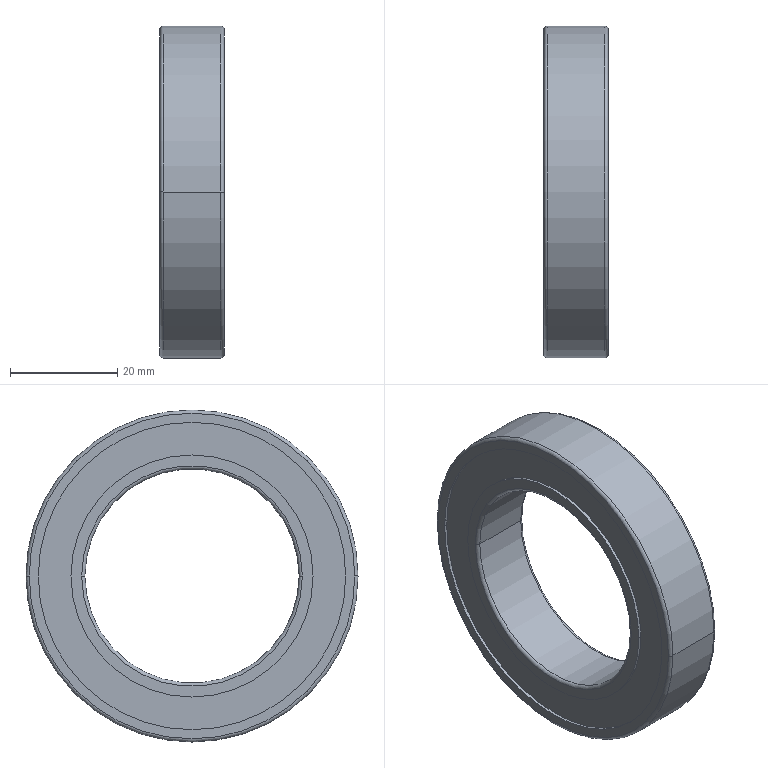Part | SolidWorks | features Fillet 2, Revolution 1 | 1 solid | 26 faces | box 12 x 62 x 62 mm | volume 20018 mm3 | cylinder 12 | torus 8 | plane 6 | commonest cylinder face diameters 45.2 x4 57.4 x4 40 x2 62 x2
STEP:
#1=CARTESIAN_POINT('',(0.6,-20.,0.));
#2=VERTEX_POINT('',#1);
#3=CARTESIAN_POINT('',(0.6,20.,0.));
#4=VERTEX_POINT('',#3);
#5=CARTESIAN_POINT('',(0.6,0.,0.));
#6=DIRECTION('',(-1.,0.,0.));
#7=DIRECTION('',(0.,1.,0.));
#8=AXIS2_PLACEMENT_3D('',#5,#6,#7);
#9=CIRCLE('',#8,20.);
#10=EDGE_CURVE('',#2,#4,#9,.T.);
#11=ORIENTED_EDGE('',*,*,#10,.F.);
#12=CARTESIAN_POINT('',(0.,-20.6,0.));
#13=VERTEX_POINT('',#12);
#14=CARTESIAN_POINT('',(0.6,-20.6,0.));
#15=DIRECTION('',(0.,0.,1.));
#16=DIRECTION('',(0.,-1.,0.));
#17=AXIS2_PLACEMENT_3D('',#14,#15,#16);
#18=CIRCLE('',#17,0.6);
#19=EDGE_CURVE('',#2,#13,#18,.T.);
#20=ORIENTED_EDGE('',*,*,#19,.T.);
#21=CARTESIAN_POINT('',(0.,20.6,0.));
#22=VERTEX_POINT('',#21);
#23=CARTESIAN_POINT('',(0.,0.,0.));
#24=DIRECTION('',(1.,0.,0.));
#25=DIRECTION('',(0.,1.,0.));
#26=AXIS2_PLACEMENT_3D('',#23,#24,#25);
#27=CIRCLE('',#26,20.6);
#28=EDGE_CURVE('',#22,#13,#27,.T.);
#29=ORIENTED_EDGE('',*,*,#28,.F.);
#30=CARTESIAN_POINT('',(0.6,20.6,0.));
#31=DIRECTION('',(0.,0.,-1.));
#32=DIRECTION('',(-1.,0.,0.));
#33=AXIS2_PLACEMENT_3D('',#30,#31,#32);
#34=CIRCLE('',#33,0.6);
#35=EDGE_CURVE('',#4,#22,#34,.T.);
#36=ORIENTED_EDGE('',*,*,#35,.F.);
#37=EDGE_LOOP('',(#11,#20,#29,#36));
#38=FACE_OUTER_BOUND('',#37,.T.);
#39=CARTESIAN_POINT('',(0.6,0.,0.));
#40=DIRECTION('',(1.,0.,0.));
#41=DIRECTION('',(0.,1.,0.));
#42=AXIS2_PLACEMENT_3D('',#39,#40,#41);
#43=TOROIDAL_SURFACE('',#42,20.6,0.6);
#44=ADVANCED_FACE('',(#38),#43,.T.);
#45=CARTESIAN_POINT('',(11.4,20.,0.));
#46=VERTEX_POINT('',#45);
#47=CARTESIAN_POINT('',(11.4,-20.,0.));
#48=VERTEX_POINT('',#47);
#49=CARTESIAN_POINT('',(11.4,0.,0.));
#50=DIRECTION('',(1.,0.,0.));
#51=DIRECTION('',(0.,-1.,0.));
#52=AXIS2_PLACEMENT_3D('',#49,#50,#51);
#53=CIRCLE('',#52,20.);
#54=EDGE_CURVE('',#46,#48,#53,.T.);
#55=ORIENTED_EDGE('',*,*,#54,.F.);
#56=CARTESIAN_POINT('',(12.,20.6,0.));
#57=VERTEX_POINT('',#56);
#58=CARTESIAN_POINT('',(11.4,20.6,0.));
#59=DIRECTION('',(0.,0.,1.));
#60=DIRECTION('',(0.,-1.,0.));
#61=AXIS2_PLACEMENT_3D('',#58,#59,#60);
#62=CIRCLE('',#61,0.6);
#63=EDGE_CURVE('',#46,#57,#62,.T.);
#64=ORIENTED_EDGE('',*,*,#63,.T.);
#65=CARTESIAN_POINT('',(12.,-20.6,0.));
#66=VERTEX_POINT('',#65);
#67=CARTESIAN_POINT('',(12.,0.,0.));
#68=DIRECTION('',(-1.,0.,0.));
#69=DIRECTION('',(0.,-1.,0.));
#70=AXIS2_PLACEMENT_3D('',#67,#68,#69);
#71=CIRCLE('',#70,20.6);
#72=EDGE_CURVE('',#66,#57,#71,.T.);
#73=ORIENTED_EDGE('',*,*,#72,.F.);
#74=CARTESIAN_POINT('',(11.4,-20.6,0.));
#75=DIRECTION('',(0.,0.,-1.));
#76=DIRECTION('',(-1.,0.,0.));
#77=AXIS2_PLACEMENT_3D('',#74,#75,#76);
#78=CIRCLE('',#77,0.6);
#79=EDGE_CURVE('',#48,#66,#78,.T.);
#80=ORIENTED_EDGE('',*,*,#79,.F.);
#81=EDGE_LOOP('',(#55,#64,#73,#80));
#82=FACE_OUTER_BOUND('',#81,.T.);
#83=CARTESIAN_POINT('',(11.4,0.,0.));
#84=DIRECTION('',(-1.,0.,0.));
#85=DIRECTION('',(0.,-1.,0.));
#86=AXIS2_PLACEMENT_3D('',#83,#84,#85);
#87=TOROIDAL_SURFACE('',#86,20.6,0.6);
#88=ADVANCED_FACE('',(#82),#87,.T.);
#89=CARTESIAN_POINT('',(0.,-30.4,0.));
#90=VERTEX_POINT('',#89);
#91=CARTESIAN_POINT('',(0.,30.4,0.));
#92=VERTEX_POINT('',#91);
#93=CARTESIAN_POINT('',(0.,0.,0.));
#94=DIRECTION('',(-1.,0.,0.));
#95=DIRECTION('',(0.,1.,0.));
#96=AXIS2_PLACEMENT_3D('',#93,#94,#95);
#97=CIRCLE('',#96,30.4);
#98=EDGE_CURVE('',#90,#92,#97,.T.);
#99=ORIENTED_EDGE('',*,*,#98,.F.);
#100=CARTESIAN_POINT('',(0.6,-31.,0.));
#101=VERTEX_POINT('',#100);
#102=CARTESIAN_POINT('',(0.6,-30.4,0.));
#103=DIRECTION('',(0.,0.,1.));
#104=DIRECTION('',(0.,-1.,0.));
#105=AXIS2_PLACEMENT_3D('',#102,#103,#104);
#106=CIRCLE('',#105,0.6);
#107=EDGE_CURVE('',#90,#101,#106,.T.);
#108=ORIENTED_EDGE('',*,*,#107,.T.);
#109=CARTESIAN_POINT('',(0.6,31.,0.));
#110=VERTEX_POINT('',#109);
#111=CARTESIAN_POINT('',(0.6,0.,0.));
#112=DIRECTION('',(1.,0.,0.));
#113=DIRECTION('',(0.,1.,0.));
#114=AXIS2_PLACEMENT_3D('',#111,#112,#113);
#115=CIRCLE('',#114,31.);
#116=EDGE_CURVE('',#110,#101,#115,.T.);
#117=ORIENTED_EDGE('',*,*,#116,.F.);
#118=CARTESIAN_POINT('',(0.6,30.4,0.));
#119=DIRECTION('',(0.,0.,-1.));
#120=DIRECTION('',(-1.,0.,0.));
#121=AXIS2_PLACEMENT_3D('',#118,#119,#120);
#122=CIRCLE('',#121,0.6);
#123=EDGE_CURVE('',#92,#110,#122,.T.);
#124=ORIENTED_EDGE('',*,*,#123,.F.);
#125=EDGE_LOOP('',(#99,#108,#117,#124));
#126=FACE_OUTER_BOUND('',#125,.T.);
#127=CARTESIAN_POINT('',(0.6,0.,0.));
#128=DIRECTION('',(1.,0.,0.));
#129=DIRECTION('',(0.,1.,0.));
#130=AXIS2_PLACEMENT_3D('',#127,#128,#129);
#131=TOROIDAL_SURFACE('',#130,30.4,0.6);
#132=ADVANCED_FACE('',(#126),#131,.T.);
#133=CARTESIAN_POINT('',(12.,30.4,0.));
#134=VERTEX_POINT('',#133);
#135=CARTESIAN_POINT('',(12.,-30.4,0.));
#136=VERTEX_POINT('',#135);
#137=CARTESIAN_POINT('',(12.,0.,0.));
#138=DIRECTION('',(1.,0.,0.));
#139=DIRECTION('',(0.,-1.,0.));
#140=AXIS2_PLACEMENT_3D('',#137,#138,#139);
#141=CIRCLE('',#140,30.4);
#142=EDGE_CURVE('',#134,#136,#141,.T.);
#143=ORIENTED_EDGE('',*,*,#142,.F.);
#144=CARTESIAN_POINT('',(11.4,31.,0.));
#145=VERTEX_POINT('',#144);
#146=CARTESIAN_POINT('',(11.4,30.4,0.));
#147=DIRECTION('',(0.,0.,1.));
#148=DIRECTION('',(0.,-1.,0.));
#149=AXIS2_PLACEMENT_3D('',#146,#147,#148);
#150=CIRCLE('',#149,0.6);
#151=EDGE_CURVE('',#134,#145,#150,.T.);
#152=ORIENTED_EDGE('',*,*,#151,.T.);
#153=CARTESIAN_POINT('',(11.4,-31.,0.));
#154=VERTEX_POINT('',#153);
#155=CARTESIAN_POINT('',(11.4,0.,0.));
#156=DIRECTION('',(-1.,0.,0.));
#157=DIRECTION('',(0.,-1.,0.));
#158=AXIS2_PLACEMENT_3D('',#155,#156,#157);
#159=CIRCLE('',#158,31.);
#160=EDGE_CURVE('',#154,#145,#159,.T.);
#161=ORIENTED_EDGE('',*,*,#160,.F.);
#162=CARTESIAN_POINT('',(11.4,-30.4,0.));
#163=DIRECTION('',(0.,0.,-1.));
#164=DIRECTION('',(-1.,0.,0.));
#165=AXIS2_PLACEMENT_3D('',#162,#163,#164);
#166=CIRCLE('',#165,0.6);
#167=EDGE_CURVE('',#136,#154,#166,.T.);
#168=ORIENTED_EDGE('',*,*,#167,.F.);
#169=EDGE_LOOP('',(#143,#152,#161,#168));
#170=FACE_OUTER_BOUND('',#169,.T.);
#171=CARTESIAN_POINT('',(11.4,0.,0.));
#172=DIRECTION('',(-1.,0.,0.));
#173=DIRECTION('',(0.,-1.,0.));
#174=AXIS2_PLACEMENT_3D('',#171,#172,#173);
#175=TOROIDAL_SURFACE('',#174,30.4,0.6);
#176=ADVANCED_FACE('',(#170),#175,.T.);
#177=ORIENTED_EDGE('',*,*,#160,.T.);
#178=CARTESIAN_POINT('',(0.,31.,0.));
#179=DIRECTION('',(-1.,0.,0.));
#180=VECTOR('',#179,1000.);
#181=LINE('',#178,#180);
#182=EDGE_CURVE('',#145,#110,#181,.T.);
#183=ORIENTED_EDGE('',*,*,#182,.T.);
#184=ORIENTED_EDGE('',*,*,#116,.T.);
#185=CARTESIAN_POINT('',(0.,-31.,0.));
#186=DIRECTION('',(-1.,0.,0.));
#187=VECTOR('',#186,1000.);
#188=LINE('',#185,#187);
#189=EDGE_CURVE('',#154,#101,#188,.T.);
#190=ORIENTED_EDGE('',*,*,#189,.F.);
#191=EDGE_LOOP('',(#177,#183,#184,#190));
#192=FACE_OUTER_BOUND('',#191,.T.);
#193=CARTESIAN_POINT('',(0.,0.,0.));
#194=DIRECTION('',(-1.,0.,0.));
#195=DIRECTION('',(0.,-1.,0.));
#196=AXIS2_PLACEMENT_3D('',#193,#194,#195);
#197=CYLINDRICAL_SURFACE('',#196,31.);
#198=ADVANCED_FACE('',(#192),#197,.T.);
#199=CARTESIAN_POINT('',(12.,28.7,0.));
#200=VERTEX_POINT('',#199);
#201=CARTESIAN_POINT('',(12.,-28.7,0.));
#202=VERTEX_POINT('',#201);
#203=CARTESIAN_POINT('',(12.,0.,0.));
#204=DIRECTION('',(-1.,0.,0.));
#205=DIRECTION('',(0.,-1.,0.));
#206=AXIS2_PLACEMENT_3D('',#203,#204,#205);
#207=CIRCLE('',#206,28.7);
#208=EDGE_CURVE('',#200,#202,#207,.T.);
#209=ORIENTED_EDGE('',*,*,#208,.F.);
#210=CARTESIAN_POINT('',(11.45,28.7,0.));
#211=VERTEX_POINT('',#210);
#212=CARTESIAN_POINT('',(0.,28.7,0.));
#213=DIRECTION('',(-1.,0.,0.));
#214=VECTOR('',#213,1000.);
#215=LINE('',#212,#214);
#216=EDGE_CURVE('',#200,#211,#215,.T.);
#217=ORIENTED_EDGE('',*,*,#216,.T.);
#218=CARTESIAN_POINT('',(11.45,-28.7,0.));
#219=VERTEX_POINT('',#218);
#220=CARTESIAN_POINT('',(11.45,0.,0.));
#221=DIRECTION('',(-1.,0.,0.));
#222=DIRECTION('',(0.,-1.,0.));
#223=AXIS2_PLACEMENT_3D('',#220,#221,#222);
#224=CIRCLE('',#223,28.7);
#225=EDGE_CURVE('',#211,#219,#224,.T.);
#226=ORIENTED_EDGE('',*,*,#225,.T.);
#227=CARTESIAN_POINT('',(0.,-28.7,0.));
#228=DIRECTION('',(-1.,0.,0.));
#229=VECTOR('',#228,1000.);
#230=LINE('',#227,#229);
#231=EDGE_CURVE('',#202,#219,#230,.T.);
#232=ORIENTED_EDGE('',*,*,#231,.F.);
#233=EDGE_LOOP('',(#209,#217,#226,#232));
#234=FACE_OUTER_BOUND('',#233,.T.);
#235=CARTESIAN_POINT('',(0.,0.,0.));
#236=DIRECTION('',(-1.,0.,0.));
#237=DIRECTION('',(0.,-1.,0.));
#238=AXIS2_PLACEMENT_3D('',#235,#236,#237);
#239=CYLINDRICAL_SURFACE('',#238,28.7);
#240=ADVANCED_FACE('',(#234),#239,.F.);
#241=CARTESIAN_POINT('',(12.,-22.6,0.));
#242=VERTEX_POINT('',#241);
#243=CARTESIAN_POINT('',(12.,22.6,0.));
#244=VERTEX_POINT('',#243);
#245=CARTESIAN_POINT('',(12.,0.,0.));
#246=DIRECTION('',(-1.,0.,0.));
#247=DIRECTION('',(0.,-1.,0.));
#248=AXIS2_PLACEMENT_3D('',#245,#246,#247);
#249=CIRCLE('',#248,22.6);
#250=EDGE_CURVE('',#242,#244,#249,.T.);
#251=ORIENTED_EDGE('',*,*,#250,.T.);
#252=CARTESIAN_POINT('',(11.45,22.6,0.));
#253=VERTEX_POINT('',#252);
#254=CARTESIAN_POINT('',(0.,22.6,0.));
#255=DIRECTION('',(-1.,0.,0.));
#256=VECTOR('',#255,1000.);
#257=LINE('',#254,#256);
#258=EDGE_CURVE('',#244,#253,#257,.T.);
#259=ORIENTED_EDGE('',*,*,#258,.T.);
#260=CARTESIAN_POINT('',(11.45,-22.6,0.));
#261=VERTEX_POINT('',#260);
#262=CARTESIAN_POINT('',(11.45,0.,0.));
#263=DIRECTION('',(-1.,0.,0.));
#264=DIRECTION('',(0.,-1.,0.));
#265=AXIS2_PLACEMENT_3D('',#262,#263,#264);
#266=CIRCLE('',#265,22.6);
#267=EDGE_CURVE('',#261,#253,#266,.T.);
#268=ORIENTED_EDGE('',*,*,#267,.F.);
#269=CARTESIAN_POINT('',(0.,-22.6,0.));
#270=DIRECTION('',(-1.,0.,0.));
#271=VECTOR('',#270,1000.);
#272=LINE('',#269,#271);
#273=EDGE_CURVE('',#242,#261,#272,.T.);
#274=ORIENTED_EDGE('',*,*,#273,.F.);
#275=EDGE_LOOP('',(#251,#259,#268,#274));
#276=FACE_OUTER_BOUND('',#275,.T.);
#277=CARTESIAN_POINT('',(0.,0.,0.));
#278=DIRECTION('',(-1.,0.,0.));
#279=DIRECTION('',(0.,-1.,0.));
#280=AXIS2_PLACEMENT_3D('',#277,#278,#279);
#281=CYLINDRICAL_SURFACE('',#280,22.6);
#282=ADVANCED_FACE('',(#276),#281,.T.);
#283=CARTESIAN_POINT('',(11.4,0.,0.));
#284=DIRECTION('',(1.,0.,0.));
#285=DIRECTION('',(0.,-1.,0.));
#286=AXIS2_PLACEMENT_3D('',#283,#284,#285);
#287=CIRCLE('',#286,20.);
#288=EDGE_CURVE('',#48,#46,#287,.T.);
#289=ORIENTED_EDGE('',*,*,#288,.T.);
#290=CARTESIAN_POINT('',(0.,20.,0.));
#291=DIRECTION('',(-1.,0.,0.));
#292=VECTOR('',#291,1000.);
#293=LINE('',#290,#292);
#294=EDGE_CURVE('',#46,#4,#293,.T.);
#295=ORIENTED_EDGE('',*,*,#294,.T.);
#296=CARTESIAN_POINT('',(0.6,0.,0.));
#297=DIRECTION('',(-1.,0.,0.));
#298=DIRECTION('',(0.,1.,0.));
#299=AXIS2_PLACEMENT_3D('',#296,#297,#298);
#300=CIRCLE('',#299,20.);
#301=EDGE_CURVE('',#4,#2,#300,.T.);
#302=ORIENTED_EDGE('',*,*,#301,.T.);
#303=CARTESIAN_POINT('',(0.,-20.,0.));
#304=DIRECTION('',(-1.,0.,0.));
#305=VECTOR('',#304,1000.);
#306=LINE('',#303,#305);
#307=EDGE_CURVE('',#48,#2,#306,.T.);
#308=ORIENTED_EDGE('',*,*,#307,.F.);
#309=EDGE_LOOP('',(#289,#295,#302,#308));
#310=FACE_OUTER_BOUND('',#309,.T.);
#311=CARTESIAN_POINT('',(0.,0.,0.));
#312=DIRECTION('',(-1.,0.,0.));
#313=DIRECTION('',(0.,-1.,0.));
#314=AXIS2_PLACEMENT_3D('',#311,#312,#313);
#315=CYLINDRICAL_SURFACE('',#314,20.);
#316=ADVANCED_FACE('',(#310),#315,.F.);
#317=CARTESIAN_POINT('',(0.55,-22.6,0.));
#318=VERTEX_POINT('',#317);
#319=CARTESIAN_POINT('',(0.55,22.6,0.));
#320=VERTEX_POINT('',#319);
#321=CARTESIAN_POINT('',(0.55,0.,0.));
#322=DIRECTION('',(-1.,0.,0.));
#323=DIRECTION('',(0.,-1.,0.));
#324=AXIS2_PLACEMENT_3D('',#321,#322,#323);
#325=CIRCLE('',#324,22.6);
#326=EDGE_CURVE('',#318,#320,#325,.T.);
#327=ORIENTED_EDGE('',*,*,#326,.T.);
#328=CARTESIAN_POINT('',(0.,22.6,0.));
#329=VERTEX_POINT('',#328);
#330=CARTESIAN_POINT('',(0.,22.6,0.));
#331=DIRECTION('',(-1.,0.,0.));
#332=VECTOR('',#331,1000.);
#333=LINE('',#330,#332);
#334=EDGE_CURVE('',#320,#329,#333,.T.);
#335=ORIENTED_EDGE('',*,*,#334,.T.);
#336=CARTESIAN_POINT('',(0.,-22.6,0.));
#337=VERTEX_POINT('',#336);
#338=CARTESIAN_POINT('',(0.,0.,0.));
#339=DIRECTION('',(-1.,0.,0.));
#340=DIRECTION('',(0.,-1.,0.));
#341=AXIS2_PLACEMENT_3D('',#338,#339,#340);
#342=CIRCLE('',#341,22.6);
#343=EDGE_CURVE('',#337,#329,#342,.T.);
#344=ORIENTED_EDGE('',*,*,#343,.F.);
#345=CARTESIAN_POINT('',(0.,-22.6,0.));
#346=DIRECTION('',(-1.,0.,0.));
#347=VECTOR('',#346,1000.);
#348=LINE('',#345,#347);
#349=EDGE_CURVE('',#318,#337,#348,.T.);
#350=ORIENTED_EDGE('',*,*,#349,.F.);
#351=EDGE_LOOP('',(#327,#335,#344,#350));
#352=FACE_OUTER_BOUND('',#351,.T.);
#353=CARTESIAN_POINT('',(0.,0.,0.));
#354=DIRECTION('',(-1.,0.,0.));
#355=DIRECTION('',(0.,-1.,0.));
#356=AXIS2_PLACEMENT_3D('',#353,#354,#355);
#357=CYLINDRICAL_SURFACE('',#356,22.6);
#358=ADVANCED_FACE('',(#352),#357,.T.);
#359=CARTESIAN_POINT('',(0.55,28.7,0.));
#360=VERTEX_POINT('',#359);
#361=CARTESIAN_POINT('',(0.55,-28.7,0.));
#362=VERTEX_POINT('',#361);
#363=CARTESIAN_POINT('',(0.55,0.,0.));
#364=DIRECTION('',(-1.,0.,0.));
#365=DIRECTION('',(0.,-1.,0.));
#366=AXIS2_PLACEMENT_3D('',#363,#364,#365);
#367=CIRCLE('',#366,28.7);
#368=EDGE_CURVE('',#360,#362,#367,.T.);
#369=ORIENTED_EDGE('',*,*,#368,.F.);
#370=CARTESIAN_POINT('',(0.,28.7,0.));
#371=VERTEX_POINT('',#370);
#372=CARTESIAN_POINT('',(0.,28.7,0.));
#373=DIRECTION('',(-1.,0.,0.));
#374=VECTOR('',#373,1000.);
#375=LINE('',#372,#374);
#376=EDGE_CURVE('',#360,#371,#375,.T.);
#377=ORIENTED_EDGE('',*,*,#376,.T.);
#378=CARTESIAN_POINT('',(0.,-28.7,0.));
#379=VERTEX_POINT('',#378);
#380=CARTESIAN_POINT('',(0.,0.,0.));
#381=DIRECTION('',(-1.,0.,0.));
#382=DIRECTION('',(0.,-1.,0.));
#383=AXIS2_PLACEMENT_3D('',#380,#381,#382);
#384=CIRCLE('',#383,28.7);
#385=EDGE_CURVE('',#371,#379,#384,.T.);
#386=ORIENTED_EDGE('',*,*,#385,.T.);
#387=CARTESIAN_POINT('',(0.,-28.7,0.));
#388=DIRECTION('',(-1.,0.,0.));
#389=VECTOR('',#388,1000.);
#390=LINE('',#387,#389);
#391=EDGE_CURVE('',#362,#379,#390,.T.);
#392=ORIENTED_EDGE('',*,*,#391,.F.);
#393=EDGE_LOOP('',(#369,#377,#386,#392));
#394=FACE_OUTER_BOUND('',#393,.T.);
#395=CARTESIAN_POINT('',(0.,0.,0.));
#396=DIRECTION('',(-1.,0.,0.));
#397=DIRECTION('',(0.,-1.,0.));
#398=AXIS2_PLACEMENT_3D('',#395,#396,#397);
#399=CYLINDRICAL_SURFACE('',#398,28.7);
#400=ADVANCED_FACE('',(#394),#399,.F.);
#401=CARTESIAN_POINT('',(0.,0.,0.));
#402=DIRECTION('',(-1.,0.,0.));
#403=DIRECTION('',(0.,1.,0.));
#404=AXIS2_PLACEMENT_3D('',#401,#402,#403);
#405=CIRCLE('',#404,30.4);
#406=EDGE_CURVE('',#92,#90,#405,.T.);
#407=ORIENTED_EDGE('',*,*,#406,.T.);
#408=ORIENTED_EDGE('',*,*,#98,.T.);
#409=EDGE_LOOP('',(#407,#408));
#410=FACE_OUTER_BOUND('',#409,.T.);
#411=CARTESIAN_POINT('',(0.,0.,0.));
#412=DIRECTION('',(-1.,0.,0.));
#413=DIRECTION('',(0.,-1.,0.));
#414=AXIS2_PLACEMENT_3D('',#411,#412,#413);
#415=CIRCLE('',#414,28.7);
#416=EDGE_CURVE('',#379,#371,#415,.T.);
#417=ORIENTED_EDGE('',*,*,#416,.F.);
#418=ORIENTED_EDGE('',*,*,#385,.F.);
#419=EDGE_LOOP('',(#417,#418));
#420=FACE_BOUND('',#419,.T.);
#421=CARTESIAN_POINT('',(0.,31.,0.));
#422=DIRECTION('',(1.,0.,0.));
#423=DIRECTION('',(0.,1.,0.));
#424=AXIS2_PLACEMENT_3D('',#421,#422,#423);
#425=PLANE('',#424);
#426=ADVANCED_FACE('',(#410,#420),#425,.F.);
#427=ORIENTED_EDGE('',*,*,#376,.F.);
#428=CARTESIAN_POINT('',(0.55,0.,0.));
#429=DIRECTION('',(-1.,0.,0.));
#430=DIRECTION('',(0.,-1.,0.));
#431=AXIS2_PLACEMENT_3D('',#428,#429,#430);
#432=CIRCLE('',#431,28.7);
#433=EDGE_CURVE('',#362,#360,#432,.T.);
#434=ORIENTED_EDGE('',*,*,#433,.F.);
#435=ORIENTED_EDGE('',*,*,#391,.T.);
#436=ORIENTED_EDGE('',*,*,#416,.T.);
#437=EDGE_LOOP('',(#427,#434,#435,#436));
#438=FACE_OUTER_BOUND('',#437,.T.);
#439=CARTESIAN_POINT('',(0.,0.,0.));
#440=DIRECTION('',(-1.,0.,0.));
#441=DIRECTION('',(0.,-1.,0.));
#442=AXIS2_PLACEMENT_3D('',#439,#440,#441);
#443=CYLINDRICAL_SURFACE('',#442,28.7);
#444=ADVANCED_FACE('',(#438),#443,.F.);
#445=ORIENTED_EDGE('',*,*,#326,.F.);
#446=CARTESIAN_POINT('',(0.55,0.,0.));
#447=DIRECTION('',(-1.,0.,0.));
#448=DIRECTION('',(0.,-1.,0.));
#449=AXIS2_PLACEMENT_3D('',#446,#447,#448);
#450=CIRCLE('',#449,22.6);
#451=EDGE_CURVE('',#320,#318,#450,.T.);
#452=ORIENTED_EDGE('',*,*,#451,.F.);
#453=EDGE_LOOP('',(#445,#452));
#454=FACE_BOUND('',#453,.T.);
#455=ORIENTED_EDGE('',*,*,#433,.T.);
#456=ORIENTED_EDGE('',*,*,#368,.T.);
#457=EDGE_LOOP('',(#455,#456));
#458=FACE_OUTER_BOUND('',#457,.T.);
#459=CARTESIAN_POINT('',(0.55,28.7,0.));
#460=DIRECTION('',(1.,0.,0.));
#461=DIRECTION('',(0.,1.,0.));
#462=AXIS2_PLACEMENT_3D('',#459,#460,#461);
#463=PLANE('',#462);
#464=ADVANCED_FACE('',(#454,#458),#463,.F.);
#465=ORIENTED_EDGE('',*,*,#334,.F.);
#466=ORIENTED_EDGE('',*,*,#451,.T.);
#467=ORIENTED_EDGE('',*,*,#349,.T.);
#468=CARTESIAN_POINT('',(0.,0.,0.));
#469=DIRECTION('',(-1.,0.,0.));
#470=DIRECTION('',(0.,-1.,0.));
#471=AXIS2_PLACEMENT_3D('',#468,#469,#470);
#472=CIRCLE('',#471,22.6);
#473=EDGE_CURVE('',#329,#337,#472,.T.);
#474=ORIENTED_EDGE('',*,*,#473,.F.);
#475=EDGE_LOOP('',(#465,#466,#467,#474));
#476=FACE_OUTER_BOUND('',#475,.T.);
#477=CARTESIAN_POINT('',(0.,0.,0.));
#478=DIRECTION('',(-1.,0.,0.));
#479=DIRECTION('',(0.,-1.,0.));
#480=AXIS2_PLACEMENT_3D('',#477,#478,#479);
#481=CYLINDRICAL_SURFACE('',#480,22.6);
#482=ADVANCED_FACE('',(#476),#481,.T.);
#483=ORIENTED_EDGE('',*,*,#28,.T.);
#484=CARTESIAN_POINT('',(0.,0.,0.));
#485=DIRECTION('',(1.,0.,0.));
#486=DIRECTION('',(0.,1.,0.));
#487=AXIS2_PLACEMENT_3D('',#484,#485,#486);
#488=CIRCLE('',#487,20.6);
#489=EDGE_CURVE('',#13,#22,#488,.T.);
#490=ORIENTED_EDGE('',*,*,#489,.T.);
#491=EDGE_LOOP('',(#483,#490));
#492=FACE_BOUND('',#491,.T.);
#493=ORIENTED_EDGE('',*,*,#343,.T.);
#494=ORIENTED_EDGE('',*,*,#473,.T.);
#495=EDGE_LOOP('',(#493,#494));
#496=FACE_OUTER_BOUND('',#495,.T.);
#497=CARTESIAN_POINT('',(0.,22.6,0.));
#498=DIRECTION('',(1.,0.,0.));
#499=DIRECTION('',(0.,1.,0.));
#500=AXIS2_PLACEMENT_3D('',#497,#498,#499);
#501=PLANE('',#500);
#502=ADVANCED_FACE('',(#492,#496),#501,.F.);
#503=ORIENTED_EDGE('',*,*,#294,.F.);
#504=ORIENTED_EDGE('',*,*,#54,.T.);
#505=ORIENTED_EDGE('',*,*,#307,.T.);
#506=ORIENTED_EDGE('',*,*,#10,.T.);
#507=EDGE_LOOP('',(#503,#504,#505,#506));
#508=FACE_OUTER_BOUND('',#507,.T.);
#509=CARTESIAN_POINT('',(0.,0.,0.));
#510=DIRECTION('',(-1.,0.,0.));
#511=DIRECTION('',(0.,-1.,0.));
#512=AXIS2_PLACEMENT_3D('',#509,#510,#511);
#513=CYLINDRICAL_SURFACE('',#512,20.);
#514=ADVANCED_FACE('',(#508),#513,.F.);
#515=ORIENTED_EDGE('',*,*,#72,.T.);
#516=CARTESIAN_POINT('',(12.,0.,0.));
#517=DIRECTION('',(-1.,0.,0.));
#518=DIRECTION('',(0.,-1.,0.));
#519=AXIS2_PLACEMENT_3D('',#516,#517,#518);
#520=CIRCLE('',#519,20.6);
#521=EDGE_CURVE('',#57,#66,#520,.T.);
#522=ORIENTED_EDGE('',*,*,#521,.T.);
#523=EDGE_LOOP('',(#515,#522));
#524=FACE_BOUND('',#523,.T.);
#525=ORIENTED_EDGE('',*,*,#250,.F.);
#526=CARTESIAN_POINT('',(12.,0.,0.));
#527=DIRECTION('',(-1.,0.,0.));
#528=DIRECTION('',(0.,-1.,0.));
#529=AXIS2_PLACEMENT_3D('',#526,#527,#528);
#530=CIRCLE('',#529,22.6);
#531=EDGE_CURVE('',#244,#242,#530,.T.);
#532=ORIENTED_EDGE('',*,*,#531,.F.);
#533=EDGE_LOOP('',(#525,#532));
#534=FACE_OUTER_BOUND('',#533,.T.);
#535=CARTESIAN_POINT('',(12.,22.6,0.));
#536=DIRECTION('',(-1.,0.,0.));
#537=DIRECTION('',(0.,-1.,0.));
#538=AXIS2_PLACEMENT_3D('',#535,#536,#537);
#539=PLANE('',#538);
#540=ADVANCED_FACE('',(#524,#534),#539,.F.);
#541=ORIENTED_EDGE('',*,*,#258,.F.);
#542=ORIENTED_EDGE('',*,*,#531,.T.);
#543=ORIENTED_EDGE('',*,*,#273,.T.);
#544=CARTESIAN_POINT('',(11.45,0.,0.));
#545=DIRECTION('',(-1.,0.,0.));
#546=DIRECTION('',(0.,-1.,0.));
#547=AXIS2_PLACEMENT_3D('',#544,#545,#546);
#548=CIRCLE('',#547,22.6);
#549=EDGE_CURVE('',#253,#261,#548,.T.);
#550=ORIENTED_EDGE('',*,*,#549,.F.);
#551=EDGE_LOOP('',(#541,#542,#543,#550));
#552=FACE_OUTER_BOUND('',#551,.T.);
#553=CARTESIAN_POINT('',(0.,0.,0.));
#554=DIRECTION('',(-1.,0.,0.));
#555=DIRECTION('',(0.,-1.,0.));
#556=AXIS2_PLACEMENT_3D('',#553,#554,#555);
#557=CYLINDRICAL_SURFACE('',#556,22.6);
#558=ADVANCED_FACE('',(#552),#557,.T.);
#559=CARTESIAN_POINT('',(11.45,0.,0.));
#560=DIRECTION('',(-1.,0.,0.));
#561=DIRECTION('',(0.,-1.,0.));
#562=AXIS2_PLACEMENT_3D('',#559,#560,#561);
#563=CIRCLE('',#562,28.7);
#564=EDGE_CURVE('',#219,#211,#563,.T.);
#565=ORIENTED_EDGE('',*,*,#564,.F.);
#566=ORIENTED_EDGE('',*,*,#225,.F.);
#567=EDGE_LOOP('',(#565,#566));
#568=FACE_OUTER_BOUND('',#567,.T.);
#569=ORIENTED_EDGE('',*,*,#267,.T.);
#570=ORIENTED_EDGE('',*,*,#549,.T.);
#571=EDGE_LOOP('',(#569,#570));
#572=FACE_BOUND('',#571,.T.);
#573=CARTESIAN_POINT('',(11.45,28.7,0.));
#574=DIRECTION('',(-1.,0.,0.));
#575=DIRECTION('',(0.,-1.,0.));
#576=AXIS2_PLACEMENT_3D('',#573,#574,#575);
#577=PLANE('',#576);
#578=ADVANCED_FACE('',(#568,#572),#577,.F.);
#579=ORIENTED_EDGE('',*,*,#216,.F.);
#580=CARTESIAN_POINT('',(12.,0.,0.));
#581=DIRECTION('',(-1.,0.,0.));
#582=DIRECTION('',(0.,-1.,0.));
#583=AXIS2_PLACEMENT_3D('',#580,#581,#582);
#584=CIRCLE('',#583,28.7);
#585=EDGE_CURVE('',#202,#200,#584,.T.);
#586=ORIENTED_EDGE('',*,*,#585,.F.);
#587=ORIENTED_EDGE('',*,*,#231,.T.);
#588=ORIENTED_EDGE('',*,*,#564,.T.);
#589=EDGE_LOOP('',(#579,#586,#587,#588));
#590=FACE_OUTER_BOUND('',#589,.T.);
#591=CARTESIAN_POINT('',(0.,0.,0.));
#592=DIRECTION('',(-1.,0.,0.));
#593=DIRECTION('',(0.,-1.,0.));
#594=AXIS2_PLACEMENT_3D('',#591,#592,#593);
#595=CYLINDRICAL_SURFACE('',#594,28.7);
#596=ADVANCED_FACE('',(#590),#595,.F.);
#597=CARTESIAN_POINT('',(12.,0.,0.));
#598=DIRECTION('',(1.,0.,0.));
#599=DIRECTION('',(0.,-1.,0.));
#600=AXIS2_PLACEMENT_3D('',#597,#598,#599);
#601=CIRCLE('',#600,30.4);
#602=EDGE_CURVE('',#136,#134,#601,.T.);
#603=ORIENTED_EDGE('',*,*,#602,.T.);
#604=ORIENTED_EDGE('',*,*,#142,.T.);
#605=EDGE_LOOP('',(#603,#604));
#606=FACE_OUTER_BOUND('',#605,.T.);
#607=ORIENTED_EDGE('',*,*,#585,.T.);
#608=ORIENTED_EDGE('',*,*,#208,.T.);
#609=EDGE_LOOP('',(#607,#608));
#610=FACE_BOUND('',#609,.T.);
#611=CARTESIAN_POINT('',(12.,31.,0.));
#612=DIRECTION('',(-1.,0.,0.));
#613=DIRECTION('',(0.,-1.,0.));
#614=AXIS2_PLACEMENT_3D('',#611,#612,#613);
#615=PLANE('',#614);
#616=ADVANCED_FACE('',(#606,#610),#615,.F.);
#617=ORIENTED_EDGE('',*,*,#182,.F.);
#618=CARTESIAN_POINT('',(11.4,0.,0.));
#619=DIRECTION('',(-1.,0.,0.));
#620=DIRECTION('',(0.,-1.,0.));
#621=AXIS2_PLACEMENT_3D('',#618,#619,#620);
#622=CIRCLE('',#621,31.);
#623=EDGE_CURVE('',#145,#154,#622,.T.);
#624=ORIENTED_EDGE('',*,*,#623,.T.);
#625=ORIENTED_EDGE('',*,*,#189,.T.);
#626=CARTESIAN_POINT('',(0.6,0.,0.));
#627=DIRECTION('',(1.,0.,0.));
#628=DIRECTION('',(0.,1.,0.));
#629=AXIS2_PLACEMENT_3D('',#626,#627,#628);
#630=CIRCLE('',#629,31.);
#631=EDGE_CURVE('',#101,#110,#630,.T.);
#632=ORIENTED_EDGE('',*,*,#631,.T.);
#633=EDGE_LOOP('',(#617,#624,#625,#632));
#634=FACE_OUTER_BOUND('',#633,.T.);
#635=CARTESIAN_POINT('',(0.,0.,0.));
#636=DIRECTION('',(-1.,0.,0.));
#637=DIRECTION('',(0.,-1.,0.));
#638=AXIS2_PLACEMENT_3D('',#635,#636,#637);
#639=CYLINDRICAL_SURFACE('',#638,31.);
#640=ADVANCED_FACE('',(#634),#639,.T.);
#641=ORIENTED_EDGE('',*,*,#151,.F.);
#642=ORIENTED_EDGE('',*,*,#602,.F.);
#643=ORIENTED_EDGE('',*,*,#167,.T.);
#644=ORIENTED_EDGE('',*,*,#623,.F.);
#645=EDGE_LOOP('',(#641,#642,#643,#644));
#646=FACE_OUTER_BOUND('',#645,.T.);
#647=CARTESIAN_POINT('',(11.4,0.,0.));
#648=DIRECTION('',(-1.,0.,0.));
#649=DIRECTION('',(0.,-1.,0.));
#650=AXIS2_PLACEMENT_3D('',#647,#648,#649);
#651=TOROIDAL_SURFACE('',#650,30.4,0.6);
#652=ADVANCED_FACE('',(#646),#651,.T.);
#653=ORIENTED_EDGE('',*,*,#107,.F.);
#654=ORIENTED_EDGE('',*,*,#406,.F.);
#655=ORIENTED_EDGE('',*,*,#123,.T.);
#656=ORIENTED_EDGE('',*,*,#631,.F.);
#657=EDGE_LOOP('',(#653,#654,#655,#656));
#658=FACE_OUTER_BOUND('',#657,.T.);
#659=CARTESIAN_POINT('',(0.6,0.,0.));
#660=DIRECTION('',(1.,0.,0.));
#661=DIRECTION('',(0.,1.,0.));
#662=AXIS2_PLACEMENT_3D('',#659,#660,#661);
#663=TOROIDAL_SURFACE('',#662,30.4,0.6);
#664=ADVANCED_FACE('',(#658),#663,.T.);
#665=ORIENTED_EDGE('',*,*,#63,.F.);
#666=ORIENTED_EDGE('',*,*,#288,.F.);
#667=ORIENTED_EDGE('',*,*,#79,.T.);
#668=ORIENTED_EDGE('',*,*,#521,.F.);
#669=EDGE_LOOP('',(#665,#666,#667,#668));
#670=FACE_OUTER_BOUND('',#669,.T.);
#671=CARTESIAN_POINT('',(11.4,0.,0.));
#672=DIRECTION('',(-1.,0.,0.));
#673=DIRECTION('',(0.,-1.,0.));
#674=AXIS2_PLACEMENT_3D('',#671,#672,#673);
#675=TOROIDAL_SURFACE('',#674,20.6,0.6);
#676=ADVANCED_FACE('',(#670),#675,.T.);
#677=ORIENTED_EDGE('',*,*,#19,.F.);
#678=ORIENTED_EDGE('',*,*,#301,.F.);
#679=ORIENTED_EDGE('',*,*,#35,.T.);
#680=ORIENTED_EDGE('',*,*,#489,.F.);
#681=EDGE_LOOP('',(#677,#678,#679,#680));
#682=FACE_OUTER_BOUND('',#681,.T.);
#683=CARTESIAN_POINT('',(0.6,0.,0.));
#684=DIRECTION('',(1.,0.,0.));
#685=DIRECTION('',(0.,1.,0.));
#686=AXIS2_PLACEMENT_3D('',#683,#684,#685);
#687=TOROIDAL_SURFACE('',#686,20.6,0.6);
#688=ADVANCED_FACE('',(#682),#687,.T.);
#689=CLOSED_SHELL('',(#44,#88,#132,#176,#198,#240,#282,#316,#358,#400,#426,#444,#464,#482,#502,#514,#540,#558,#578,#596,#616,#640,#652,#664,#676,#688));
#690=MANIFOLD_SOLID_BREP('',#689);
#691=CARTESIAN_POINT('',(0.,0.,0.));
#692=DIRECTION('',(0.,0.,1.));
#693=DIRECTION('',(1.,0.,0.));
#694=AXIS2_PLACEMENT_3D('',#691,#692,#693);
#695=(LENGTH_UNIT()NAMED_UNIT(*)SI_UNIT(.MILLI.,.METRE.));
#696=UNCERTAINTY_MEASURE_WITH_UNIT(LENGTH_MEASURE(0.00001),#695,'','');
#697=(NAMED_UNIT(*)PLANE_ANGLE_UNIT()SI_UNIT($,.RADIAN.));
#698=(NAMED_UNIT(*)SI_UNIT($,.STERADIAN.)SOLID_ANGLE_UNIT());
#699=(GEOMETRIC_REPRESENTATION_CONTEXT(3)GLOBAL_UNCERTAINTY_ASSIGNED_CONTEXT((#696))GLOBAL_UNIT_ASSIGNED_CONTEXT((#695,#697,#698))REPRESENTATION_CONTEXT('',''));
#700=ADVANCED_BREP_SHAPE_REPRESENTATION('',(#690,#694),#699);